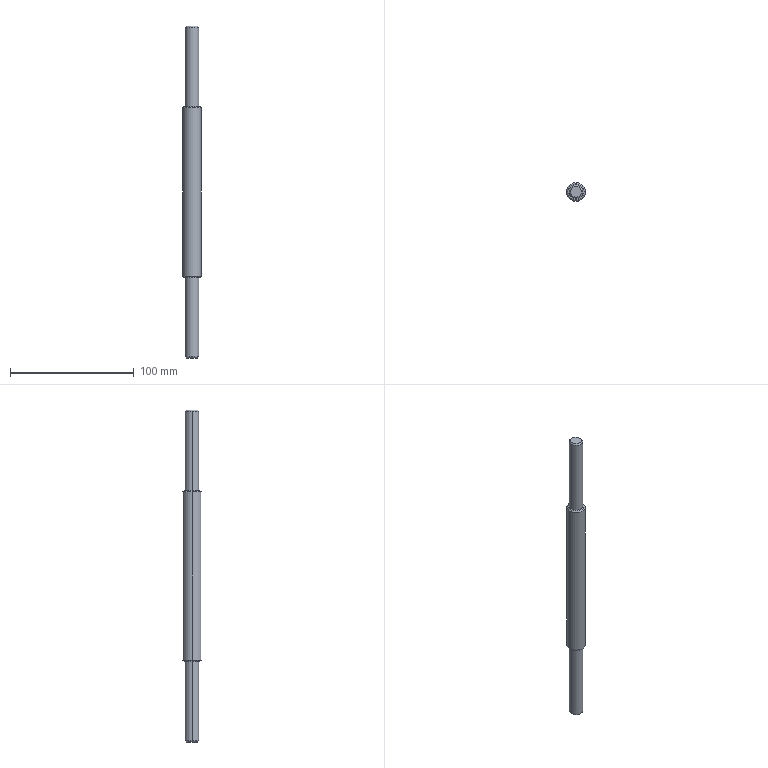Part | SolidWorks | features ICE 3, Chamfer 2, Extrusion 1 | 1 solid | 18 faces | box 15 x 15 x 268 mm | volume 36663 mm3 | cone 8 | cylinder 6 | plane 4 | commonest cylinder face diameters 11 x4 15 x2
STEP:
#1=CARTESIAN_POINT('',(-4.5,0.,-65.));
#2=VERTEX_POINT('',#1);
#3=CARTESIAN_POINT('',(4.5,0.,-65.));
#4=VERTEX_POINT('',#3);
#5=CARTESIAN_POINT('',(0.,0.,-65.));
#6=DIRECTION('',(0.,0.,-1.));
#7=DIRECTION('',(-1.,0.,0.));
#8=AXIS2_PLACEMENT_3D('',#5,#6,#7);
#9=CIRCLE('',#8,4.5);
#10=EDGE_CURVE('',#2,#4,#9,.T.);
#11=ORIENTED_EDGE('',*,*,#10,.F.);
#12=CARTESIAN_POINT('',(-5.5,0.,-64.));
#13=VERTEX_POINT('',#12);
#14=CARTESIAN_POINT('',(-4.5,0.,-65.));
#15=DIRECTION('',(-0.7071,0.,0.7071));
#16=VECTOR('',#15,1000.);
#17=LINE('',#14,#16);
#18=EDGE_CURVE('',#2,#13,#17,.T.);
#19=ORIENTED_EDGE('',*,*,#18,.T.);
#20=CARTESIAN_POINT('',(5.5,0.,-64.));
#21=VERTEX_POINT('',#20);
#22=CARTESIAN_POINT('',(0.,0.,-64.));
#23=DIRECTION('',(0.,0.,1.));
#24=DIRECTION('',(-1.,0.,0.));
#25=AXIS2_PLACEMENT_3D('',#22,#23,#24);
#26=CIRCLE('',#25,5.5);
#27=EDGE_CURVE('',#21,#13,#26,.T.);
#28=ORIENTED_EDGE('',*,*,#27,.F.);
#29=CARTESIAN_POINT('',(4.5,0.,-65.));
#30=DIRECTION('',(0.7071,0.,0.7071));
#31=VECTOR('',#30,1000.);
#32=LINE('',#29,#31);
#33=EDGE_CURVE('',#4,#21,#32,.T.);
#34=ORIENTED_EDGE('',*,*,#33,.F.);
#35=EDGE_LOOP('',(#11,#19,#28,#34));
#36=FACE_OUTER_BOUND('',#35,.T.);
#37=CARTESIAN_POINT('',(0.,0.,-65.));
#38=DIRECTION('',(0.,0.,1.));
#39=DIRECTION('',(1.,0.,0.));
#40=AXIS2_PLACEMENT_3D('',#37,#38,#39);
#41=CONICAL_SURFACE('',#40,4.5,0.7854);
#42=ADVANCED_FACE('',(#36),#41,.T.);
#43=ORIENTED_EDGE('',*,*,#27,.T.);
#44=CARTESIAN_POINT('',(-5.5,0.,0.));
#45=VERTEX_POINT('',#44);
#46=CARTESIAN_POINT('',(-5.5,0.,-65.));
#47=DIRECTION('',(0.,0.,1.));
#48=VECTOR('',#47,1000.);
#49=LINE('',#46,#48);
#50=EDGE_CURVE('',#13,#45,#49,.T.);
#51=ORIENTED_EDGE('',*,*,#50,.T.);
#52=CARTESIAN_POINT('',(5.5,0.,0.));
#53=VERTEX_POINT('',#52);
#54=CARTESIAN_POINT('',(0.,0.,0.));
#55=DIRECTION('',(0.,0.,-1.));
#56=DIRECTION('',(1.,0.,0.));
#57=AXIS2_PLACEMENT_3D('',#54,#55,#56);
#58=CIRCLE('',#57,5.5);
#59=EDGE_CURVE('',#45,#53,#58,.T.);
#60=ORIENTED_EDGE('',*,*,#59,.T.);
#61=CARTESIAN_POINT('',(5.5,0.,-65.));
#62=DIRECTION('',(0.,0.,1.));
#63=VECTOR('',#62,1000.);
#64=LINE('',#61,#63);
#65=EDGE_CURVE('',#21,#53,#64,.T.);
#66=ORIENTED_EDGE('',*,*,#65,.F.);
#67=EDGE_LOOP('',(#43,#51,#60,#66));
#68=FACE_OUTER_BOUND('',#67,.T.);
#69=CARTESIAN_POINT('',(0.,0.,-65.));
#70=DIRECTION('',(0.,0.,1.));
#71=DIRECTION('',(1.,0.,0.));
#72=AXIS2_PLACEMENT_3D('',#69,#70,#71);
#73=CYLINDRICAL_SURFACE('',#72,5.5);
#74=ADVANCED_FACE('',(#68),#73,.T.);
#75=CARTESIAN_POINT('',(6.5,0.,138.));
#76=VERTEX_POINT('',#75);
#77=CARTESIAN_POINT('',(-6.5,0.,138.));
#78=VERTEX_POINT('',#77);
#79=CARTESIAN_POINT('',(0.,0.,138.));
#80=DIRECTION('',(0.,0.,1.));
#81=DIRECTION('',(1.,0.,0.));
#82=AXIS2_PLACEMENT_3D('',#79,#80,#81);
#83=CIRCLE('',#82,6.5);
#84=EDGE_CURVE('',#76,#78,#83,.T.);
#85=ORIENTED_EDGE('',*,*,#84,.F.);
#86=CARTESIAN_POINT('',(7.5,0.,137.));
#87=VERTEX_POINT('',#86);
#88=CARTESIAN_POINT('',(6.5,0.,138.));
#89=DIRECTION('',(0.7071,0.,-0.7071));
#90=VECTOR('',#89,1000.);
#91=LINE('',#88,#90);
#92=EDGE_CURVE('',#76,#87,#91,.T.);
#93=ORIENTED_EDGE('',*,*,#92,.T.);
#94=CARTESIAN_POINT('',(-7.5,0.,137.));
#95=VERTEX_POINT('',#94);
#96=CARTESIAN_POINT('',(0.,0.,137.));
#97=DIRECTION('',(0.,0.,-1.));
#98=DIRECTION('',(1.,0.,0.));
#99=AXIS2_PLACEMENT_3D('',#96,#97,#98);
#100=CIRCLE('',#99,7.5);
#101=EDGE_CURVE('',#95,#87,#100,.T.);
#102=ORIENTED_EDGE('',*,*,#101,.F.);
#103=CARTESIAN_POINT('',(-6.5,0.,138.));
#104=DIRECTION('',(-0.7071,0.,-0.7071));
#105=VECTOR('',#104,1000.);
#106=LINE('',#103,#105);
#107=EDGE_CURVE('',#78,#95,#106,.T.);
#108=ORIENTED_EDGE('',*,*,#107,.F.);
#109=EDGE_LOOP('',(#85,#93,#102,#108));
#110=FACE_OUTER_BOUND('',#109,.T.);
#111=CARTESIAN_POINT('',(0.,0.,138.));
#112=DIRECTION('',(0.,0.,-1.));
#113=DIRECTION('',(-1.,0.,0.));
#114=AXIS2_PLACEMENT_3D('',#111,#112,#113);
#115=CONICAL_SURFACE('',#114,6.5,0.7854);
#116=ADVANCED_FACE('',(#110),#115,.T.);
#117=CARTESIAN_POINT('',(-6.5,0.,0.));
#118=VERTEX_POINT('',#117);
#119=CARTESIAN_POINT('',(6.5,0.,0.));
#120=VERTEX_POINT('',#119);
#121=CARTESIAN_POINT('',(0.,0.,0.));
#122=DIRECTION('',(0.,0.,-1.));
#123=DIRECTION('',(1.,0.,0.));
#124=AXIS2_PLACEMENT_3D('',#121,#122,#123);
#125=CIRCLE('',#124,6.5);
#126=EDGE_CURVE('',#118,#120,#125,.T.);
#127=ORIENTED_EDGE('',*,*,#126,.F.);
#128=CARTESIAN_POINT('',(-7.5,0.,1.));
#129=VERTEX_POINT('',#128);
#130=CARTESIAN_POINT('',(-7.5,0.,1.));
#131=DIRECTION('',(-0.7071,0.,0.7071));
#132=VECTOR('',#131,1000.);
#133=LINE('',#130,#132);
#134=EDGE_CURVE('',#118,#129,#133,.T.);
#135=ORIENTED_EDGE('',*,*,#134,.T.);
#136=CARTESIAN_POINT('',(7.5,0.,1.));
#137=VERTEX_POINT('',#136);
#138=CARTESIAN_POINT('',(0.,0.,1.));
#139=DIRECTION('',(0.,0.,1.));
#140=DIRECTION('',(1.,0.,0.));
#141=AXIS2_PLACEMENT_3D('',#138,#139,#140);
#142=CIRCLE('',#141,7.5);
#143=EDGE_CURVE('',#137,#129,#142,.T.);
#144=ORIENTED_EDGE('',*,*,#143,.F.);
#145=CARTESIAN_POINT('',(7.5,0.,1.));
#146=DIRECTION('',(0.7071,0.,0.7071));
#147=VECTOR('',#146,1000.);
#148=LINE('',#145,#147);
#149=EDGE_CURVE('',#120,#137,#148,.T.);
#150=ORIENTED_EDGE('',*,*,#149,.F.);
#151=EDGE_LOOP('',(#127,#135,#144,#150));
#152=FACE_OUTER_BOUND('',#151,.T.);
#153=CARTESIAN_POINT('',(0.,0.,1.));
#154=DIRECTION('',(0.,0.,1.));
#155=DIRECTION('',(1.,0.,0.));
#156=AXIS2_PLACEMENT_3D('',#153,#154,#155);
#157=CONICAL_SURFACE('',#156,7.5,0.7854);
#158=ADVANCED_FACE('',(#152),#157,.T.);
#159=CARTESIAN_POINT('',(4.5,0.,203.));
#160=VERTEX_POINT('',#159);
#161=CARTESIAN_POINT('',(-4.5,0.,203.));
#162=VERTEX_POINT('',#161);
#163=CARTESIAN_POINT('',(0.,0.,203.));
#164=DIRECTION('',(0.,0.,1.));
#165=DIRECTION('',(1.,0.,0.));
#166=AXIS2_PLACEMENT_3D('',#163,#164,#165);
#167=CIRCLE('',#166,4.5);
#168=EDGE_CURVE('',#160,#162,#167,.T.);
#169=ORIENTED_EDGE('',*,*,#168,.F.);
#170=CARTESIAN_POINT('',(5.5,0.,202.));
#171=VERTEX_POINT('',#170);
#172=CARTESIAN_POINT('',(4.5,0.,203.));
#173=DIRECTION('',(0.7071,0.,-0.7071));
#174=VECTOR('',#173,1000.);
#175=LINE('',#172,#174);
#176=EDGE_CURVE('',#160,#171,#175,.T.);
#177=ORIENTED_EDGE('',*,*,#176,.T.);
#178=CARTESIAN_POINT('',(-5.5,0.,202.));
#179=VERTEX_POINT('',#178);
#180=CARTESIAN_POINT('',(0.,0.,202.));
#181=DIRECTION('',(0.,0.,-1.));
#182=DIRECTION('',(1.,0.,0.));
#183=AXIS2_PLACEMENT_3D('',#180,#181,#182);
#184=CIRCLE('',#183,5.5);
#185=EDGE_CURVE('',#179,#171,#184,.T.);
#186=ORIENTED_EDGE('',*,*,#185,.F.);
#187=CARTESIAN_POINT('',(-4.5,0.,203.));
#188=DIRECTION('',(-0.7071,0.,-0.7071));
#189=VECTOR('',#188,1000.);
#190=LINE('',#187,#189);
#191=EDGE_CURVE('',#162,#179,#190,.T.);
#192=ORIENTED_EDGE('',*,*,#191,.F.);
#193=EDGE_LOOP('',(#169,#177,#186,#192));
#194=FACE_OUTER_BOUND('',#193,.T.);
#195=CARTESIAN_POINT('',(0.,0.,203.));
#196=DIRECTION('',(0.,0.,-1.));
#197=DIRECTION('',(-1.,0.,0.));
#198=AXIS2_PLACEMENT_3D('',#195,#196,#197);
#199=CONICAL_SURFACE('',#198,4.5,0.7854);
#200=ADVANCED_FACE('',(#194),#199,.T.);
#201=ORIENTED_EDGE('',*,*,#185,.T.);
#202=CARTESIAN_POINT('',(5.5,0.,138.));
#203=VERTEX_POINT('',#202);
#204=CARTESIAN_POINT('',(5.5,0.,158.));
#205=DIRECTION('',(0.,0.,-1.));
#206=VECTOR('',#205,1000.);
#207=LINE('',#204,#206);
#208=EDGE_CURVE('',#171,#203,#207,.T.);
#209=ORIENTED_EDGE('',*,*,#208,.T.);
#210=CARTESIAN_POINT('',(-5.5,0.,138.));
#211=VERTEX_POINT('',#210);
#212=CARTESIAN_POINT('',(0.,0.,138.));
#213=DIRECTION('',(0.,0.,1.));
#214=DIRECTION('',(1.,0.,0.));
#215=AXIS2_PLACEMENT_3D('',#212,#213,#214);
#216=CIRCLE('',#215,5.5);
#217=EDGE_CURVE('',#203,#211,#216,.T.);
#218=ORIENTED_EDGE('',*,*,#217,.T.);
#219=CARTESIAN_POINT('',(-5.5,0.,158.));
#220=DIRECTION('',(0.,0.,-1.));
#221=VECTOR('',#220,1000.);
#222=LINE('',#219,#221);
#223=EDGE_CURVE('',#179,#211,#222,.T.);
#224=ORIENTED_EDGE('',*,*,#223,.F.);
#225=EDGE_LOOP('',(#201,#209,#218,#224));
#226=FACE_OUTER_BOUND('',#225,.T.);
#227=CARTESIAN_POINT('',(0.,0.,158.));
#228=DIRECTION('',(0.,0.,-1.));
#229=DIRECTION('',(-1.,0.,0.));
#230=AXIS2_PLACEMENT_3D('',#227,#228,#229);
#231=CYLINDRICAL_SURFACE('',#230,5.5);
#232=ADVANCED_FACE('',(#226),#231,.T.);
#233=ORIENTED_EDGE('',*,*,#101,.T.);
#234=CARTESIAN_POINT('',(7.5,0.,138.));
#235=DIRECTION('',(0.,0.,-1.));
#236=VECTOR('',#235,1000.);
#237=LINE('',#234,#236);
#238=EDGE_CURVE('',#87,#137,#237,.T.);
#239=ORIENTED_EDGE('',*,*,#238,.T.);
#240=ORIENTED_EDGE('',*,*,#143,.T.);
#241=CARTESIAN_POINT('',(-7.5,0.,138.));
#242=DIRECTION('',(0.,0.,-1.));
#243=VECTOR('',#242,1000.);
#244=LINE('',#241,#243);
#245=EDGE_CURVE('',#95,#129,#244,.T.);
#246=ORIENTED_EDGE('',*,*,#245,.F.);
#247=EDGE_LOOP('',(#233,#239,#240,#246));
#248=FACE_OUTER_BOUND('',#247,.T.);
#249=CARTESIAN_POINT('',(0.,0.,138.));
#250=DIRECTION('',(0.,0.,-1.));
#251=DIRECTION('',(-1.,0.,0.));
#252=AXIS2_PLACEMENT_3D('',#249,#250,#251);
#253=CYLINDRICAL_SURFACE('',#252,7.5);
#254=ADVANCED_FACE('',(#248),#253,.T.);
#255=CARTESIAN_POINT('',(0.,0.,0.));
#256=DIRECTION('',(0.,0.,-1.));
#257=DIRECTION('',(1.,0.,0.));
#258=AXIS2_PLACEMENT_3D('',#255,#256,#257);
#259=CIRCLE('',#258,6.5);
#260=EDGE_CURVE('',#120,#118,#259,.T.);
#261=ORIENTED_EDGE('',*,*,#260,.T.);
#262=ORIENTED_EDGE('',*,*,#126,.T.);
#263=EDGE_LOOP('',(#261,#262));
#264=FACE_OUTER_BOUND('',#263,.T.);
#265=CARTESIAN_POINT('',(0.,0.,0.));
#266=DIRECTION('',(0.,0.,-1.));
#267=DIRECTION('',(1.,0.,0.));
#268=AXIS2_PLACEMENT_3D('',#265,#266,#267);
#269=CIRCLE('',#268,5.5);
#270=EDGE_CURVE('',#53,#45,#269,.T.);
#271=ORIENTED_EDGE('',*,*,#270,.F.);
#272=ORIENTED_EDGE('',*,*,#59,.F.);
#273=EDGE_LOOP('',(#271,#272));
#274=FACE_BOUND('',#273,.T.);
#275=CARTESIAN_POINT('',(0.,0.,0.));
#276=DIRECTION('',(0.,0.,1.));
#277=DIRECTION('',(1.,0.,0.));
#278=AXIS2_PLACEMENT_3D('',#275,#276,#277);
#279=PLANE('',#278);
#280=ADVANCED_FACE('',(#264,#274),#279,.F.);
#281=CARTESIAN_POINT('',(0.,0.,138.));
#282=DIRECTION('',(0.,0.,1.));
#283=DIRECTION('',(1.,0.,0.));
#284=AXIS2_PLACEMENT_3D('',#281,#282,#283);
#285=CIRCLE('',#284,6.5);
#286=EDGE_CURVE('',#78,#76,#285,.T.);
#287=ORIENTED_EDGE('',*,*,#286,.T.);
#288=ORIENTED_EDGE('',*,*,#84,.T.);
#289=EDGE_LOOP('',(#287,#288));
#290=FACE_OUTER_BOUND('',#289,.T.);
#291=CARTESIAN_POINT('',(0.,0.,138.));
#292=DIRECTION('',(0.,0.,1.));
#293=DIRECTION('',(1.,0.,0.));
#294=AXIS2_PLACEMENT_3D('',#291,#292,#293);
#295=CIRCLE('',#294,5.5);
#296=EDGE_CURVE('',#211,#203,#295,.T.);
#297=ORIENTED_EDGE('',*,*,#296,.F.);
#298=ORIENTED_EDGE('',*,*,#217,.F.);
#299=EDGE_LOOP('',(#297,#298));
#300=FACE_BOUND('',#299,.T.);
#301=CARTESIAN_POINT('',(0.,0.,138.));
#302=DIRECTION('',(0.,0.,1.));
#303=DIRECTION('',(1.,0.,0.));
#304=AXIS2_PLACEMENT_3D('',#301,#302,#303);
#305=PLANE('',#304);
#306=ADVANCED_FACE('',(#290,#300),#305,.T.);
#307=ORIENTED_EDGE('',*,*,#238,.F.);
#308=CARTESIAN_POINT('',(0.,0.,137.));
#309=DIRECTION('',(0.,0.,-1.));
#310=DIRECTION('',(1.,0.,0.));
#311=AXIS2_PLACEMENT_3D('',#308,#309,#310);
#312=CIRCLE('',#311,7.5);
#313=EDGE_CURVE('',#87,#95,#312,.T.);
#314=ORIENTED_EDGE('',*,*,#313,.T.);
#315=ORIENTED_EDGE('',*,*,#245,.T.);
#316=CARTESIAN_POINT('',(0.,0.,1.));
#317=DIRECTION('',(0.,0.,1.));
#318=DIRECTION('',(1.,0.,0.));
#319=AXIS2_PLACEMENT_3D('',#316,#317,#318);
#320=CIRCLE('',#319,7.5);
#321=EDGE_CURVE('',#129,#137,#320,.T.);
#322=ORIENTED_EDGE('',*,*,#321,.T.);
#323=EDGE_LOOP('',(#307,#314,#315,#322));
#324=FACE_OUTER_BOUND('',#323,.T.);
#325=CARTESIAN_POINT('',(0.,0.,138.));
#326=DIRECTION('',(0.,0.,-1.));
#327=DIRECTION('',(-1.,0.,0.));
#328=AXIS2_PLACEMENT_3D('',#325,#326,#327);
#329=CYLINDRICAL_SURFACE('',#328,7.5);
#330=ADVANCED_FACE('',(#324),#329,.T.);
#331=ORIENTED_EDGE('',*,*,#208,.F.);
#332=CARTESIAN_POINT('',(0.,0.,202.));
#333=DIRECTION('',(0.,0.,-1.));
#334=DIRECTION('',(1.,0.,0.));
#335=AXIS2_PLACEMENT_3D('',#332,#333,#334);
#336=CIRCLE('',#335,5.5);
#337=EDGE_CURVE('',#171,#179,#336,.T.);
#338=ORIENTED_EDGE('',*,*,#337,.T.);
#339=ORIENTED_EDGE('',*,*,#223,.T.);
#340=ORIENTED_EDGE('',*,*,#296,.T.);
#341=EDGE_LOOP('',(#331,#338,#339,#340));
#342=FACE_OUTER_BOUND('',#341,.T.);
#343=CARTESIAN_POINT('',(0.,0.,158.));
#344=DIRECTION('',(0.,0.,-1.));
#345=DIRECTION('',(-1.,0.,0.));
#346=AXIS2_PLACEMENT_3D('',#343,#344,#345);
#347=CYLINDRICAL_SURFACE('',#346,5.5);
#348=ADVANCED_FACE('',(#342),#347,.T.);
#349=CARTESIAN_POINT('',(0.,0.,203.));
#350=DIRECTION('',(0.,0.,1.));
#351=DIRECTION('',(1.,0.,0.));
#352=AXIS2_PLACEMENT_3D('',#349,#350,#351);
#353=CIRCLE('',#352,4.5);
#354=EDGE_CURVE('',#162,#160,#353,.T.);
#355=ORIENTED_EDGE('',*,*,#354,.T.);
#356=ORIENTED_EDGE('',*,*,#168,.T.);
#357=EDGE_LOOP('',(#355,#356));
#358=FACE_OUTER_BOUND('',#357,.T.);
#359=CARTESIAN_POINT('',(0.,0.,203.));
#360=DIRECTION('',(0.,0.,1.));
#361=DIRECTION('',(1.,0.,0.));
#362=AXIS2_PLACEMENT_3D('',#359,#360,#361);
#363=PLANE('',#362);
#364=ADVANCED_FACE('',(#358),#363,.T.);
#365=ORIENTED_EDGE('',*,*,#176,.F.);
#366=ORIENTED_EDGE('',*,*,#354,.F.);
#367=ORIENTED_EDGE('',*,*,#191,.T.);
#368=ORIENTED_EDGE('',*,*,#337,.F.);
#369=EDGE_LOOP('',(#365,#366,#367,#368));
#370=FACE_OUTER_BOUND('',#369,.T.);
#371=CARTESIAN_POINT('',(0.,0.,203.));
#372=DIRECTION('',(0.,0.,-1.));
#373=DIRECTION('',(-1.,0.,0.));
#374=AXIS2_PLACEMENT_3D('',#371,#372,#373);
#375=CONICAL_SURFACE('',#374,4.5,0.7854);
#376=ADVANCED_FACE('',(#370),#375,.T.);
#377=ORIENTED_EDGE('',*,*,#134,.F.);
#378=ORIENTED_EDGE('',*,*,#260,.F.);
#379=ORIENTED_EDGE('',*,*,#149,.T.);
#380=ORIENTED_EDGE('',*,*,#321,.F.);
#381=EDGE_LOOP('',(#377,#378,#379,#380));
#382=FACE_OUTER_BOUND('',#381,.T.);
#383=CARTESIAN_POINT('',(0.,0.,1.));
#384=DIRECTION('',(0.,0.,1.));
#385=DIRECTION('',(1.,0.,0.));
#386=AXIS2_PLACEMENT_3D('',#383,#384,#385);
#387=CONICAL_SURFACE('',#386,7.5,0.7854);
#388=ADVANCED_FACE('',(#382),#387,.T.);
#389=ORIENTED_EDGE('',*,*,#92,.F.);
#390=ORIENTED_EDGE('',*,*,#286,.F.);
#391=ORIENTED_EDGE('',*,*,#107,.T.);
#392=ORIENTED_EDGE('',*,*,#313,.F.);
#393=EDGE_LOOP('',(#389,#390,#391,#392));
#394=FACE_OUTER_BOUND('',#393,.T.);
#395=CARTESIAN_POINT('',(0.,0.,138.));
#396=DIRECTION('',(0.,0.,-1.));
#397=DIRECTION('',(-1.,0.,0.));
#398=AXIS2_PLACEMENT_3D('',#395,#396,#397);
#399=CONICAL_SURFACE('',#398,6.5,0.7854);
#400=ADVANCED_FACE('',(#394),#399,.T.);
#401=ORIENTED_EDGE('',*,*,#50,.F.);
#402=CARTESIAN_POINT('',(0.,0.,-64.));
#403=DIRECTION('',(0.,0.,1.));
#404=DIRECTION('',(-1.,0.,0.));
#405=AXIS2_PLACEMENT_3D('',#402,#403,#404);
#406=CIRCLE('',#405,5.5);
#407=EDGE_CURVE('',#13,#21,#406,.T.);
#408=ORIENTED_EDGE('',*,*,#407,.T.);
#409=ORIENTED_EDGE('',*,*,#65,.T.);
#410=ORIENTED_EDGE('',*,*,#270,.T.);
#411=EDGE_LOOP('',(#401,#408,#409,#410));
#412=FACE_OUTER_BOUND('',#411,.T.);
#413=CARTESIAN_POINT('',(0.,0.,-65.));
#414=DIRECTION('',(0.,0.,1.));
#415=DIRECTION('',(1.,0.,0.));
#416=AXIS2_PLACEMENT_3D('',#413,#414,#415);
#417=CYLINDRICAL_SURFACE('',#416,5.5);
#418=ADVANCED_FACE('',(#412),#417,.T.);
#419=CARTESIAN_POINT('',(0.,0.,-65.));
#420=DIRECTION('',(0.,0.,-1.));
#421=DIRECTION('',(-1.,0.,0.));
#422=AXIS2_PLACEMENT_3D('',#419,#420,#421);
#423=CIRCLE('',#422,4.5);
#424=EDGE_CURVE('',#4,#2,#423,.T.);
#425=ORIENTED_EDGE('',*,*,#424,.T.);
#426=ORIENTED_EDGE('',*,*,#10,.T.);
#427=EDGE_LOOP('',(#425,#426));
#428=FACE_OUTER_BOUND('',#427,.T.);
#429=CARTESIAN_POINT('',(0.,0.,-65.));
#430=DIRECTION('',(0.,0.,-1.));
#431=DIRECTION('',(-1.,0.,0.));
#432=AXIS2_PLACEMENT_3D('',#429,#430,#431);
#433=PLANE('',#432);
#434=ADVANCED_FACE('',(#428),#433,.T.);
#435=ORIENTED_EDGE('',*,*,#18,.F.);
#436=ORIENTED_EDGE('',*,*,#424,.F.);
#437=ORIENTED_EDGE('',*,*,#33,.T.);
#438=ORIENTED_EDGE('',*,*,#407,.F.);
#439=EDGE_LOOP('',(#435,#436,#437,#438));
#440=FACE_OUTER_BOUND('',#439,.T.);
#441=CARTESIAN_POINT('',(0.,0.,-65.));
#442=DIRECTION('',(0.,0.,1.));
#443=DIRECTION('',(1.,0.,0.));
#444=AXIS2_PLACEMENT_3D('',#441,#442,#443);
#445=CONICAL_SURFACE('',#444,4.5,0.7854);
#446=ADVANCED_FACE('',(#440),#445,.T.);
#447=CLOSED_SHELL('',(#42,#74,#116,#158,#200,#232,#254,#280,#306,#330,#348,#364,#376,#388,#400,#418,#434,#446));
#448=MANIFOLD_SOLID_BREP('',#447);
#449=CARTESIAN_POINT('',(0.,0.,0.));
#450=DIRECTION('',(0.,0.,1.));
#451=DIRECTION('',(1.,0.,0.));
#452=AXIS2_PLACEMENT_3D('',#449,#450,#451);
#453=(LENGTH_UNIT()NAMED_UNIT(*)SI_UNIT(.MILLI.,.METRE.));
#454=UNCERTAINTY_MEASURE_WITH_UNIT(LENGTH_MEASURE(0.00001),#453,'','');
#455=(NAMED_UNIT(*)PLANE_ANGLE_UNIT()SI_UNIT($,.RADIAN.));
#456=(NAMED_UNIT(*)SI_UNIT($,.STERADIAN.)SOLID_ANGLE_UNIT());
#457=(GEOMETRIC_REPRESENTATION_CONTEXT(3)GLOBAL_UNCERTAINTY_ASSIGNED_CONTEXT((#454))GLOBAL_UNIT_ASSIGNED_CONTEXT((#453,#455,#456))REPRESENTATION_CONTEXT('',''));
#458=ADVANCED_BREP_SHAPE_REPRESENTATION('',(#448,#452),#457);